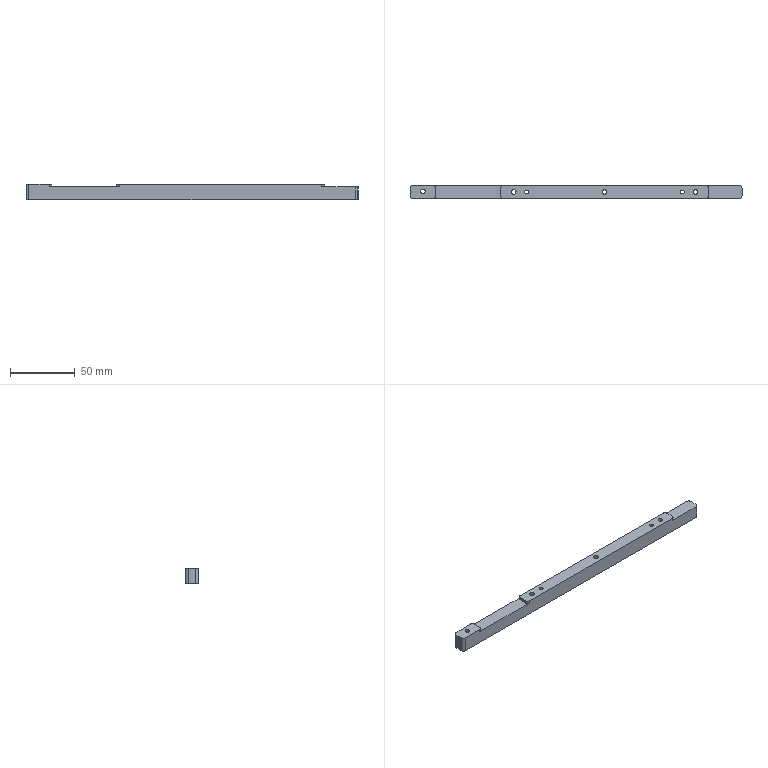Part | STEP file | ASND-0110-PWP TOP tu pang 20130814.sldasm-Part-1aq | 1 solid | 48 faces | box 256 x 10 x 12 mm | volume 28147 mm3 | cylinder 32 | plane 16 | commonest cylinder face diameters 4 x12 3.5 x8 6 x8 3 x4